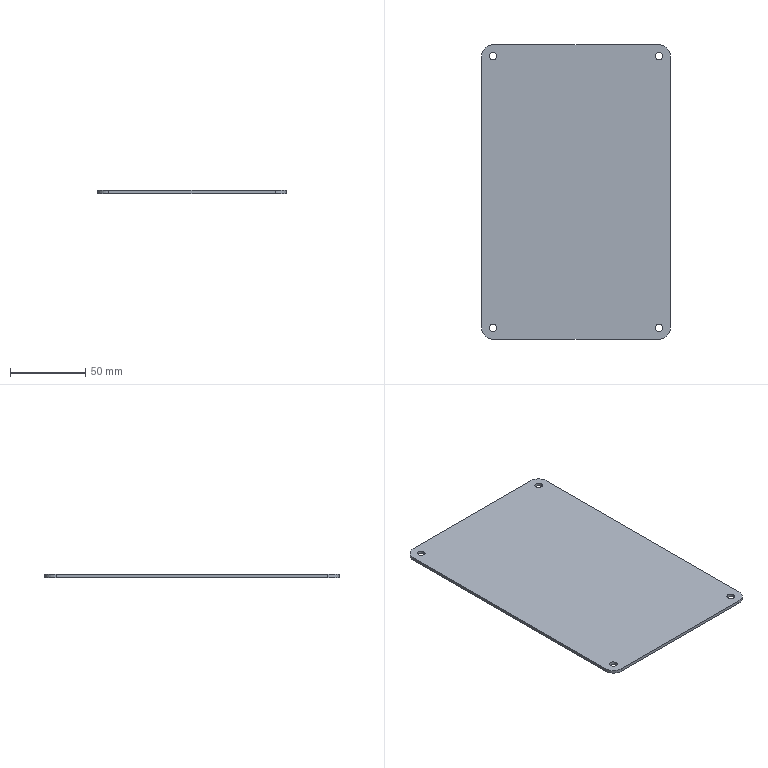Part | STEP file | Mimic panel | 1 solid | 404 faces | box 125 x 195 x 2 mm | volume 47954 mm3 | plane 346 | cylinder 58 | commonest cylinder face diameters 3.767 x12 4.567 x12 5 x8 8.455 x7 9.255 x7 10 x4